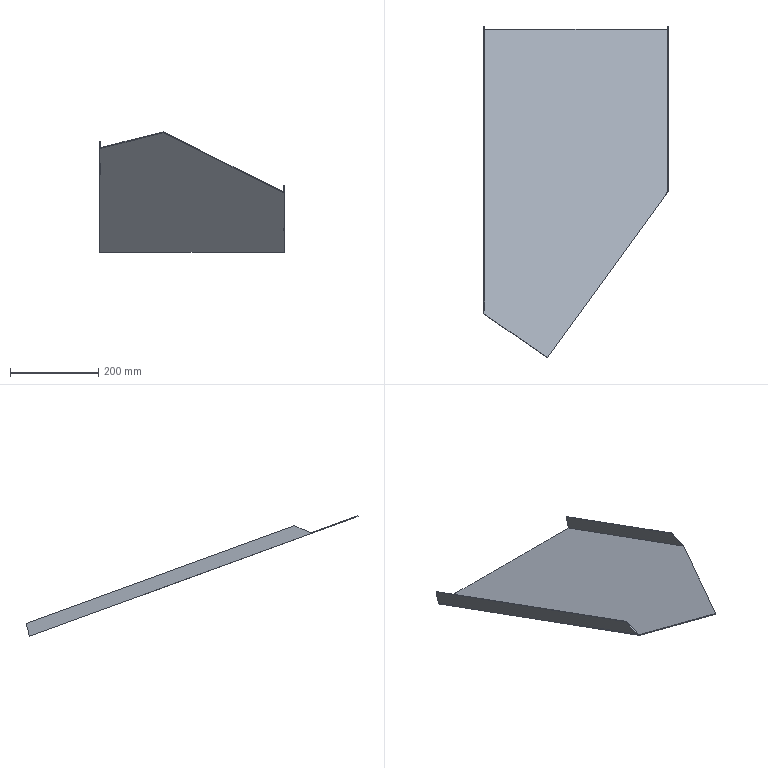Part | NX | features solid 2 | 1 solid | 13 faces | box 418.583 x 752.314 x 272.863 mm | volume 592956 mm3 | plane 12 | spline 1
STEP:
#1=CARTESIAN_POINT('',(-905.1,748.985,-499.373));
#2=VERTEX_POINT('',#1);
#3=CARTESIAN_POINT('',(-490.517,748.985,-499.373));
#4=VERTEX_POINT('',#3);
#5=CARTESIAN_POINT('',(-752.3,748.985,-499.373));
#6=DIRECTION('',(1.,0.,0.));
#7=VECTOR('',#6,1000.);
#8=LINE('',#5,#7);
#9=EDGE_CURVE('',#2,#4,#8,.T.);
#10=ORIENTED_EDGE('',*,*,#9,.F.);
#11=CARTESIAN_POINT('',(-905.1,111.413,-267.316));
#12=VERTEX_POINT('',#11);
#13=CARTESIAN_POINT('',(-905.1,3.724,-228.121));
#14=DIRECTION('',(0.,0.9397,-0.342));
#15=VECTOR('',#14,1000.);
#16=LINE('',#13,#15);
#17=EDGE_CURVE('',#12,#2,#16,.T.);
#18=ORIENTED_EDGE('',*,*,#17,.F.);
#19=CARTESIAN_POINT('',(-907.1,111.413,-267.316));
#20=VERTEX_POINT('',#19);
#21=CARTESIAN_POINT('',(-917.1,111.413,-267.316));
#22=DIRECTION('',(1.,0.,0.));
#23=VECTOR('',#22,1000.);
#24=LINE('',#21,#23);
#25=EDGE_CURVE('',#12,#20,#24,.F.);
#26=ORIENTED_EDGE('',*,*,#25,.T.);
#27=CARTESIAN_POINT('',(-907.1,104.555,-264.82));
#28=VERTEX_POINT('',#27);
#29=CARTESIAN_POINT('',(-907.1,3.724,-228.121));
#30=DIRECTION('',(0.,-0.9397,0.342));
#31=VECTOR('',#30,1000.);
#32=LINE('',#29,#31);
#33=EDGE_CURVE('',#20,#28,#32,.T.);
#34=ORIENTED_EDGE('',*,*,#33,.T.);
#35=CARTESIAN_POINT('',(-762.353,4.629,-228.45));
#36=VERTEX_POINT('',#35);
#37=CARTESIAN_POINT('',(-907.1,104.555,-264.82));
#38=CARTESIAN_POINT('',(-896.947,97.59,-262.285));
#39=CARTESIAN_POINT('',(-883.394,88.293,-258.901));
#40=CARTESIAN_POINT('',(-868.677,78.196,-255.226));
#41=CARTESIAN_POINT('',(-859.316,71.771,-252.888));
#42=CARTESIAN_POINT('',(-851.631,66.496,-250.968));
#43=CARTESIAN_POINT('',(-846.624,63.058,-249.716));
#44=CARTESIAN_POINT('',(-843.853,61.154,-249.023));
#45=CARTESIAN_POINT('',(-842.479,60.21,-248.68));
#46=CARTESIAN_POINT('',(-841.553,59.573,-248.448));
#47=CARTESIAN_POINT('',(-840.869,59.103,-248.277));
#48=CARTESIAN_POINT('',(-840.374,58.762,-248.153));
#49=CARTESIAN_POINT('',(-840.088,58.565,-248.081));
#50=CARTESIAN_POINT('',(-839.869,58.414,-248.026));
#51=CARTESIAN_POINT('',(-839.743,58.327,-247.994));
#52=CARTESIAN_POINT('',(-839.635,58.253,-247.967));
#53=CARTESIAN_POINT('',(-839.583,58.217,-247.954));
#54=CARTESIAN_POINT('',(-839.237,57.979,-247.868));
#55=CARTESIAN_POINT('',(-838.878,57.732,-247.778));
#56=CARTESIAN_POINT('',(-838.395,57.399,-247.656));
#57=CARTESIAN_POINT('',(-837.64,56.879,-247.467));
#58=CARTESIAN_POINT('',(-836.689,56.223,-247.229));
#59=CARTESIAN_POINT('',(-835.549,55.437,-246.943));
#60=CARTESIAN_POINT('',(-834.026,54.387,-246.56));
#61=CARTESIAN_POINT('',(-831.356,52.545,-245.89));
#62=CARTESIAN_POINT('',(-827.525,49.9,-244.927));
#63=CARTESIAN_POINT('',(-822.904,46.706,-243.765));
#64=CARTESIAN_POINT('',(-818.257,43.491,-242.595));
#65=CARTESIAN_POINT('',(-813.586,40.256,-241.417));
#66=CARTESIAN_POINT('',(-809.672,37.543,-240.43));
#67=CARTESIAN_POINT('',(-806.921,35.635,-239.735));
#68=CARTESIAN_POINT('',(-805.347,34.542,-239.337));
#69=CARTESIAN_POINT('',(-804.162,33.72,-239.038));
#70=CARTESIAN_POINT('',(-802.985,32.903,-238.741));
#71=CARTESIAN_POINT('',(-801.974,32.2,-238.485));
#72=CARTESIAN_POINT('',(-801.322,31.748,-238.32));
#73=CARTESIAN_POINT('',(-800.861,31.427,-238.204));
#74=CARTESIAN_POINT('',(-800.879,31.44,-238.208));
#75=CARTESIAN_POINT('',(-800.728,31.335,-238.17));
#76=CARTESIAN_POINT('',(-800.56,31.218,-238.127));
#77=CARTESIAN_POINT('',(-800.282,31.025,-238.057));
#78=CARTESIAN_POINT('',(-799.781,30.676,-237.93));
#79=CARTESIAN_POINT('',(-799.007,30.138,-237.735));
#80=CARTESIAN_POINT('',(-797.857,29.338,-237.443));
#81=CARTESIAN_POINT('',(-796.021,28.061,-236.978));
#82=CARTESIAN_POINT('',(-793.163,26.073,-236.255));
#83=CARTESIAN_POINT('',(-788.833,23.059,-235.158));
#84=CARTESIAN_POINT('',(-783.602,19.419,-233.833));
#85=CARTESIAN_POINT('',(-775.426,13.729,-231.762));
#86=CARTESIAN_POINT('',(-767.943,8.52,-229.866));
#87=CARTESIAN_POINT('',(-762.353,4.629,-228.45));
#88=B_SPLINE_CURVE_WITH_KNOTS('',3,(#37,#38,#39,#40,#41,#42,#43,#44,#45,#46,#47,#48,#49,#50,#51,#52,#53,#54,#55,#56,#57,#58,#59,#60,#61,#62,#63,#64,#65,#66,#67,#68,#69,#70,#71,#72,#73,#74,#75,#76,#77,#78,#79,#80,#81,#82,#83,#84,#85,#86,#87),.UNSPECIFIED.,.F.,.F.,(4,1,1,1,1,1,1,1,1,1,1,1,1,1,1,1,1,1,1,1,1,1,1,1,1,1,1,1,1,1,1,1,1,1,1,1,1,1,1,1,1,1,1,1,1,1,1,1,4),(0.03814,0.1584,0.2185,0.2786,0.3387,0.3988,0.4289,0.4439,0.459,0.474,0.4815,0.489,0.4928,0.4965,0.4984,0.5003,0.5022,0.504,0.5078,0.5116,0.5191,0.5266,0.5341,0.5491,0.5792,0.6092,0.6393,0.6694,0.6994,0.7144,0.722,0.7295,0.737,0.7445,0.7483,0.7501,0.752,0.7558,0.7595,0.767,0.7746,0.7896,0.8046,0.8197,0.8497,0.8798,0.9098,0.9399,1.),.UNSPECIFIED.);
#89=EDGE_CURVE('',#28,#36,#88,.T.);
#90=ORIENTED_EDGE('',*,*,#89,.T.);
#91=CARTESIAN_POINT('',(-488.517,382.431,-365.958));
#92=VERTEX_POINT('',#91);
#93=CARTESIAN_POINT('',(-846.744,-111.802,-186.072));
#94=DIRECTION('',(0.5629,0.7767,-0.2827));
#95=VECTOR('',#94,1000.);
#96=LINE('',#93,#95);
#97=EDGE_CURVE('',#92,#36,#96,.F.);
#98=ORIENTED_EDGE('',*,*,#97,.F.);
#99=CARTESIAN_POINT('',(-490.517,382.431,-365.958));
#100=VERTEX_POINT('',#99);
#101=CARTESIAN_POINT('',(-488.517,382.431,-365.958));
#102=DIRECTION('',(-1.,0.,0.));
#103=VECTOR('',#102,1000.);
#104=LINE('',#101,#103);
#105=EDGE_CURVE('',#92,#100,#104,.T.);
#106=ORIENTED_EDGE('',*,*,#105,.T.);
#107=CARTESIAN_POINT('',(-490.517,3.724,-228.121));
#108=DIRECTION('',(0.,0.9397,-0.342));
#109=VECTOR('',#108,1000.);
#110=LINE('',#107,#109);
#111=EDGE_CURVE('',#100,#4,#110,.T.);
#112=ORIENTED_EDGE('',*,*,#111,.T.);
#113=EDGE_LOOP('',(#10,#18,#26,#34,#90,#98,#106,#112));
#114=FACE_BOUND('',#113,.T.);
#115=CARTESIAN_POINT('',(-752.3,3.724,-228.121));
#116=DIRECTION('',(0.,0.342,0.9397));
#117=DIRECTION('',(1.,0.,0.));
#118=AXIS2_PLACEMENT_3D('',#115,#116,#117);
#119=PLANE('',#118);
#120=ADVANCED_FACE('',(#114),#119,.T.);
#121=CARTESIAN_POINT('',(-488.517,756.26,-472.224));
#122=VERTEX_POINT('',#121);
#123=CARTESIAN_POINT('',(-488.517,748.465,-501.312));
#124=VERTEX_POINT('',#123);
#125=CARTESIAN_POINT('',(-488.517,766.359,-434.531));
#126=DIRECTION('',(0.,-0.2588,-0.9659));
#127=VECTOR('',#126,1000.);
#128=LINE('',#125,#127);
#129=EDGE_CURVE('',#122,#124,#128,.T.);
#130=ORIENTED_EDGE('',*,*,#129,.F.);
#131=CARTESIAN_POINT('',(-488.517,418.318,-349.224));
#132=VERTEX_POINT('',#131);
#133=CARTESIAN_POINT('',(-488.517,392.007,-339.647));
#134=DIRECTION('',(0.,0.9397,-0.342));
#135=VECTOR('',#134,1000.);
#136=LINE('',#133,#135);
#137=EDGE_CURVE('',#132,#122,#136,.T.);
#138=ORIENTED_EDGE('',*,*,#137,.F.);
#139=CARTESIAN_POINT('',(-488.517,381.149,-366.556));
#140=DIRECTION('',(0.,0.9063,0.4226));
#141=VECTOR('',#140,1000.);
#142=LINE('',#139,#141);
#143=EDGE_CURVE('',#132,#92,#142,.F.);
#144=ORIENTED_EDGE('',*,*,#143,.T.);
#145=CARTESIAN_POINT('',(-488.517,381.746,-367.838));
#146=VERTEX_POINT('',#145);
#147=CARTESIAN_POINT('',(-488.517,381.746,-367.838));
#148=DIRECTION('',(0.,0.342,0.9397));
#149=VECTOR('',#148,1000.);
#150=LINE('',#147,#149);
#151=EDGE_CURVE('',#146,#92,#150,.T.);
#152=ORIENTED_EDGE('',*,*,#151,.F.);
#153=CARTESIAN_POINT('',(-488.517,3.04,-230.));
#154=DIRECTION('',(0.,0.9397,-0.342));
#155=VECTOR('',#154,1000.);
#156=LINE('',#153,#155);
#157=EDGE_CURVE('',#146,#124,#156,.T.);
#158=ORIENTED_EDGE('',*,*,#157,.T.);
#159=EDGE_LOOP('',(#130,#138,#144,#152,#158));
#160=FACE_BOUND('',#159,.T.);
#161=CARTESIAN_POINT('',(-488.517,3.04,-230.));
#162=DIRECTION('',(1.,0.,0.));
#163=DIRECTION('',(0.,1.,0.));
#164=AXIS2_PLACEMENT_3D('',#161,#162,#163);
#165=PLANE('',#164);
#166=ADVANCED_FACE('',(#160),#165,.T.);
#167=CARTESIAN_POINT('',(-907.1,147.301,-250.581));
#168=VERTEX_POINT('',#167);
#169=CARTESIAN_POINT('',(-907.1,756.26,-472.224));
#170=VERTEX_POINT('',#169);
#171=CARTESIAN_POINT('',(-907.1,120.99,-241.005));
#172=DIRECTION('',(0.,-0.9397,0.342));
#173=VECTOR('',#172,1000.);
#174=LINE('',#171,#173);
#175=EDGE_CURVE('',#168,#170,#174,.F.);
#176=ORIENTED_EDGE('',*,*,#175,.T.);
#177=CARTESIAN_POINT('',(-907.1,748.465,-501.312));
#178=VERTEX_POINT('',#177);
#179=CARTESIAN_POINT('',(-907.1,766.359,-434.531));
#180=DIRECTION('',(0.,-0.2588,-0.9659));
#181=VECTOR('',#180,1000.);
#182=LINE('',#179,#181);
#183=EDGE_CURVE('',#170,#178,#182,.T.);
#184=ORIENTED_EDGE('',*,*,#183,.T.);
#185=CARTESIAN_POINT('',(-907.1,103.871,-266.699));
#186=VERTEX_POINT('',#185);
#187=CARTESIAN_POINT('',(-907.1,3.04,-230.));
#188=DIRECTION('',(0.,0.9397,-0.342));
#189=VECTOR('',#188,1000.);
#190=LINE('',#187,#189);
#191=EDGE_CURVE('',#186,#178,#190,.T.);
#192=ORIENTED_EDGE('',*,*,#191,.F.);
#193=CARTESIAN_POINT('',(-907.1,104.213,-265.759));
#194=DIRECTION('',(0.,0.342,0.9397));
#195=VECTOR('',#194,1000.);
#196=LINE('',#193,#195);
#197=EDGE_CURVE('',#186,#28,#196,.T.);
#198=ORIENTED_EDGE('',*,*,#197,.T.);
#199=ORIENTED_EDGE('',*,*,#33,.F.);
#200=CARTESIAN_POINT('',(-907.1,147.301,-250.581));
#201=DIRECTION('',(0.,-0.9063,-0.4226));
#202=VECTOR('',#201,1000.);
#203=LINE('',#200,#202);
#204=EDGE_CURVE('',#20,#168,#203,.F.);
#205=ORIENTED_EDGE('',*,*,#204,.T.);
#206=EDGE_LOOP('',(#176,#184,#192,#198,#199,#205));
#207=FACE_BOUND('',#206,.T.);
#208=CARTESIAN_POINT('',(-907.1,3.04,-230.));
#209=DIRECTION('',(1.,0.,0.));
#210=DIRECTION('',(0.,0.,-1.));
#211=AXIS2_PLACEMENT_3D('',#208,#209,#210);
#212=PLANE('',#211);
#213=ADVANCED_FACE('',(#207),#212,.F.);
#214=ORIENTED_EDGE('',*,*,#89,.F.);
#215=ORIENTED_EDGE('',*,*,#197,.F.);
#216=CARTESIAN_POINT('',(-762.353,3.945,-230.329));
#217=VERTEX_POINT('',#216);
#218=CARTESIAN_POINT('',(-907.1,103.871,-266.699));
#219=CARTESIAN_POINT('',(-896.947,96.906,-264.164));
#220=CARTESIAN_POINT('',(-883.394,87.609,-260.781));
#221=CARTESIAN_POINT('',(-868.677,77.512,-257.105));
#222=CARTESIAN_POINT('',(-859.316,71.087,-254.767));
#223=CARTESIAN_POINT('',(-851.631,65.812,-252.847));
#224=CARTESIAN_POINT('',(-846.624,62.374,-251.596));
#225=CARTESIAN_POINT('',(-843.853,60.47,-250.903));
#226=CARTESIAN_POINT('',(-842.479,59.526,-250.559));
#227=CARTESIAN_POINT('',(-841.553,58.889,-250.327));
#228=CARTESIAN_POINT('',(-840.869,58.419,-250.156));
#229=CARTESIAN_POINT('',(-840.374,58.078,-250.032));
#230=CARTESIAN_POINT('',(-840.088,57.881,-249.96));
#231=CARTESIAN_POINT('',(-839.869,57.73,-249.906));
#232=CARTESIAN_POINT('',(-839.743,57.643,-249.874));
#233=CARTESIAN_POINT('',(-839.635,57.569,-249.847));
#234=CARTESIAN_POINT('',(-839.583,57.533,-249.834));
#235=CARTESIAN_POINT('',(-839.237,57.295,-249.747));
#236=CARTESIAN_POINT('',(-838.878,57.048,-249.657));
#237=CARTESIAN_POINT('',(-838.395,56.715,-249.536));
#238=CARTESIAN_POINT('',(-837.64,56.194,-249.347));
#239=CARTESIAN_POINT('',(-836.689,55.539,-249.108));
#240=CARTESIAN_POINT('',(-835.549,54.753,-248.822));
#241=CARTESIAN_POINT('',(-834.026,53.703,-248.44));
#242=CARTESIAN_POINT('',(-831.356,51.861,-247.769));
#243=CARTESIAN_POINT('',(-827.525,49.216,-246.807));
#244=CARTESIAN_POINT('',(-822.904,46.022,-245.644));
#245=CARTESIAN_POINT('',(-818.257,42.807,-244.474));
#246=CARTESIAN_POINT('',(-813.586,39.572,-243.296));
#247=CARTESIAN_POINT('',(-809.672,36.859,-242.309));
#248=CARTESIAN_POINT('',(-806.921,34.951,-241.614));
#249=CARTESIAN_POINT('',(-805.347,33.858,-241.217));
#250=CARTESIAN_POINT('',(-804.162,33.036,-240.917));
#251=CARTESIAN_POINT('',(-802.985,32.219,-240.62));
#252=CARTESIAN_POINT('',(-801.974,31.516,-240.364));
#253=CARTESIAN_POINT('',(-801.322,31.064,-240.2));
#254=CARTESIAN_POINT('',(-800.861,30.743,-240.083));
#255=CARTESIAN_POINT('',(-800.879,30.756,-240.088));
#256=CARTESIAN_POINT('',(-800.728,30.651,-240.049));
#257=CARTESIAN_POINT('',(-800.56,30.534,-240.007));
#258=CARTESIAN_POINT('',(-800.282,30.341,-239.937));
#259=CARTESIAN_POINT('',(-799.781,29.992,-239.81));
#260=CARTESIAN_POINT('',(-799.007,29.454,-239.614));
#261=CARTESIAN_POINT('',(-797.857,28.654,-239.323));
#262=CARTESIAN_POINT('',(-796.021,27.377,-238.858));
#263=CARTESIAN_POINT('',(-793.163,25.389,-238.134));
#264=CARTESIAN_POINT('',(-788.833,22.375,-237.037));
#265=CARTESIAN_POINT('',(-783.602,18.735,-235.712));
#266=CARTESIAN_POINT('',(-775.426,13.045,-233.641));
#267=CARTESIAN_POINT('',(-767.943,7.836,-231.745));
#268=CARTESIAN_POINT('',(-762.353,3.945,-230.329));
#269=B_SPLINE_CURVE_WITH_KNOTS('',3,(#218,#219,#220,#221,#222,#223,#224,#225,#226,#227,#228,#229,#230,#231,#232,#233,#234,#235,#236,#237,#238,#239,#240,#241,#242,#243,#244,#245,#246,#247,#248,#249,#250,#251,#252,#253,#254,#255,#256,#257,#258,#259,#260,#261,#262,#263,#264,#265,#266,#267,#268),.UNSPECIFIED.,.F.,.F.,(4,1,1,1,1,1,1,1,1,1,1,1,1,1,1,1,1,1,1,1,1,1,1,1,1,1,1,1,1,1,1,1,1,1,1,1,1,1,1,1,1,1,1,1,1,1,1,1,4),(0.03814,0.1584,0.2185,0.2786,0.3387,0.3988,0.4289,0.4439,0.459,0.474,0.4815,0.489,0.4928,0.4965,0.4984,0.5003,0.5022,0.504,0.5078,0.5116,0.5191,0.5266,0.5341,0.5491,0.5792,0.6092,0.6393,0.6694,0.6994,0.7144,0.722,0.7295,0.737,0.7445,0.7483,0.7501,0.752,0.7558,0.7595,0.767,0.7746,0.7896,0.8046,0.8197,0.8497,0.8798,0.9098,0.9399,1.),.UNSPECIFIED.);
#270=EDGE_CURVE('',#186,#217,#269,.T.);
#271=ORIENTED_EDGE('',*,*,#270,.T.);
#272=CARTESIAN_POINT('',(-762.353,3.945,-230.329));
#273=CARTESIAN_POINT('',(-762.353,4.173,-229.703));
#274=CARTESIAN_POINT('',(-762.353,4.401,-229.076));
#275=CARTESIAN_POINT('',(-762.353,4.629,-228.45));
#276=B_SPLINE_CURVE_WITH_KNOTS('',3,(#272,#273,#274,#275),.UNSPECIFIED.,.F.,.F.,(4,4),(0.,1.),.UNSPECIFIED.);
#277=EDGE_CURVE('',#217,#36,#276,.T.);
#278=ORIENTED_EDGE('',*,*,#277,.T.);
#279=EDGE_LOOP('',(#214,#215,#271,#278));
#280=FACE_BOUND('',#279,.T.);
#281=CARTESIAN_POINT('',(-907.1,103.871,-266.699));
#282=CARTESIAN_POINT('',(-907.1,104.555,-264.82));
#283=CARTESIAN_POINT('',(-886.794,89.942,-261.63));
#284=CARTESIAN_POINT('',(-886.794,90.626,-259.75));
#285=CARTESIAN_POINT('',(-867.,76.362,-256.687));
#286=CARTESIAN_POINT('',(-867.,77.047,-254.808));
#287=CARTESIAN_POINT('',(-851.631,65.812,-252.847));
#288=CARTESIAN_POINT('',(-851.631,66.496,-250.968));
#289=CARTESIAN_POINT('',(-846.624,62.374,-251.596));
#290=CARTESIAN_POINT('',(-846.624,63.058,-249.716));
#291=CARTESIAN_POINT('',(-843.853,60.47,-250.903));
#292=CARTESIAN_POINT('',(-843.853,61.154,-249.023));
#293=CARTESIAN_POINT('',(-842.479,59.526,-250.559));
#294=CARTESIAN_POINT('',(-842.479,60.21,-248.68));
#295=CARTESIAN_POINT('',(-841.553,58.889,-250.327));
#296=CARTESIAN_POINT('',(-841.553,59.573,-248.448));
#297=CARTESIAN_POINT('',(-840.869,58.419,-250.156));
#298=CARTESIAN_POINT('',(-840.869,59.103,-248.277));
#299=CARTESIAN_POINT('',(-840.374,58.078,-250.032));
#300=CARTESIAN_POINT('',(-840.374,58.762,-248.153));
#301=CARTESIAN_POINT('',(-840.088,57.881,-249.96));
#302=CARTESIAN_POINT('',(-840.088,58.565,-248.081));
#303=CARTESIAN_POINT('',(-839.869,57.73,-249.906));
#304=CARTESIAN_POINT('',(-839.869,58.414,-248.026));
#305=CARTESIAN_POINT('',(-839.743,57.643,-249.874));
#306=CARTESIAN_POINT('',(-839.743,58.327,-247.994));
#307=CARTESIAN_POINT('',(-839.635,57.569,-249.847));
#308=CARTESIAN_POINT('',(-839.635,58.253,-247.967));
#309=CARTESIAN_POINT('',(-839.583,57.533,-249.834));
#310=CARTESIAN_POINT('',(-839.583,58.217,-247.954));
#311=CARTESIAN_POINT('',(-839.237,57.295,-249.747));
#312=CARTESIAN_POINT('',(-839.237,57.979,-247.868));
#313=CARTESIAN_POINT('',(-838.878,57.048,-249.657));
#314=CARTESIAN_POINT('',(-838.878,57.732,-247.778));
#315=CARTESIAN_POINT('',(-838.395,56.715,-249.536));
#316=CARTESIAN_POINT('',(-838.395,57.399,-247.656));
#317=CARTESIAN_POINT('',(-837.64,56.194,-249.347));
#318=CARTESIAN_POINT('',(-837.64,56.879,-247.467));
#319=CARTESIAN_POINT('',(-836.689,55.539,-249.108));
#320=CARTESIAN_POINT('',(-836.689,56.223,-247.229));
#321=CARTESIAN_POINT('',(-835.549,54.753,-248.822));
#322=CARTESIAN_POINT('',(-835.549,55.437,-246.943));
#323=CARTESIAN_POINT('',(-834.026,53.703,-248.44));
#324=CARTESIAN_POINT('',(-834.026,54.387,-246.56));
#325=CARTESIAN_POINT('',(-831.356,51.861,-247.769));
#326=CARTESIAN_POINT('',(-831.356,52.545,-245.89));
#327=CARTESIAN_POINT('',(-825.993,48.158,-246.422));
#328=CARTESIAN_POINT('',(-825.993,48.842,-244.542));
#329=CARTESIAN_POINT('',(-819.814,43.886,-244.867));
#330=CARTESIAN_POINT('',(-819.814,44.57,-242.987));
#331=CARTESIAN_POINT('',(-813.586,39.572,-243.296));
#332=CARTESIAN_POINT('',(-813.586,40.256,-241.417));
#333=CARTESIAN_POINT('',(-809.672,36.859,-242.309));
#334=CARTESIAN_POINT('',(-809.672,37.543,-240.43));
#335=CARTESIAN_POINT('',(-806.921,34.951,-241.614));
#336=CARTESIAN_POINT('',(-806.921,35.635,-239.735));
#337=CARTESIAN_POINT('',(-805.347,33.858,-241.217));
#338=CARTESIAN_POINT('',(-805.347,34.542,-239.337));
#339=CARTESIAN_POINT('',(-804.162,33.036,-240.917));
#340=CARTESIAN_POINT('',(-804.162,33.72,-239.038));
#341=CARTESIAN_POINT('',(-802.985,32.219,-240.62));
#342=CARTESIAN_POINT('',(-802.985,32.903,-238.741));
#343=CARTESIAN_POINT('',(-801.974,31.516,-240.364));
#344=CARTESIAN_POINT('',(-801.974,32.2,-238.485));
#345=CARTESIAN_POINT('',(-801.322,31.064,-240.2));
#346=CARTESIAN_POINT('',(-801.322,31.748,-238.32));
#347=CARTESIAN_POINT('',(-800.861,30.743,-240.083));
#348=CARTESIAN_POINT('',(-800.861,31.427,-238.204));
#349=CARTESIAN_POINT('',(-800.879,30.756,-240.088));
#350=CARTESIAN_POINT('',(-800.879,31.44,-238.208));
#351=CARTESIAN_POINT('',(-800.728,30.651,-240.049));
#352=CARTESIAN_POINT('',(-800.728,31.335,-238.17));
#353=CARTESIAN_POINT('',(-800.56,30.534,-240.007));
#354=CARTESIAN_POINT('',(-800.56,31.218,-238.127));
#355=CARTESIAN_POINT('',(-800.282,30.341,-239.937));
#356=CARTESIAN_POINT('',(-800.282,31.025,-238.057));
#357=CARTESIAN_POINT('',(-799.781,29.992,-239.81));
#358=CARTESIAN_POINT('',(-799.781,30.676,-237.93));
#359=CARTESIAN_POINT('',(-799.007,29.454,-239.614));
#360=CARTESIAN_POINT('',(-799.007,30.138,-237.735));
#361=CARTESIAN_POINT('',(-797.857,28.654,-239.323));
#362=CARTESIAN_POINT('',(-797.857,29.338,-237.443));
#363=CARTESIAN_POINT('',(-796.021,27.377,-238.858));
#364=CARTESIAN_POINT('',(-796.021,28.061,-236.978));
#365=CARTESIAN_POINT('',(-793.163,25.389,-238.134));
#366=CARTESIAN_POINT('',(-793.163,26.073,-236.255));
#367=CARTESIAN_POINT('',(-788.833,22.375,-237.037));
#368=CARTESIAN_POINT('',(-788.833,23.059,-235.158));
#369=CARTESIAN_POINT('',(-783.602,18.735,-235.712));
#370=CARTESIAN_POINT('',(-783.602,19.419,-233.833));
#371=CARTESIAN_POINT('',(-775.426,13.045,-233.641));
#372=CARTESIAN_POINT('',(-775.426,13.729,-231.762));
#373=CARTESIAN_POINT('',(-767.943,7.836,-231.745));
#374=CARTESIAN_POINT('',(-767.943,8.52,-229.866));
#375=CARTESIAN_POINT('',(-762.353,3.945,-230.329));
#376=CARTESIAN_POINT('',(-762.353,4.629,-228.45));
#377=B_SPLINE_SURFACE_WITH_KNOTS('',3,1,((#281,#282),(#283,#284),(#285,#286),(#287,#288),(#289,#290),(#291,#292),(#293,#294),(#295,#296),(#297,#298),(#299,#300),(#301,#302),(#303,#304),(#305,#306),(#307,#308),(#309,#310),(#311,#312),(#313,#314),(#315,#316),(#317,#318),(#319,#320),(#321,#322),(#323,#324),(#325,#326),(#327,#328),(#329,#330),(#331,#332),(#333,#334),(#335,#336),(#337,#338),(#339,#340),(#341,#342),(#343,#344),(#345,#346),(#347,#348),(#349,#350),(#351,#352),(#353,#354),(#355,#356),(#357,#358),(#359,#360),(#361,#362),(#363,#364),(#365,#366),(#367,#368),(#369,#370),(#371,#372),(#373,#374),(#375,#376)),.UNSPECIFIED.,.F.,.F.,.F.,(4,1,1,1,1,1,1,1,1,1,1,1,1,1,1,1,1,1,1,1,1,1,1,1,1,1,1,1,1,1,1,1,1,1,1,1,1,1,1,1,1,1,1,1,1,4),(2,2),(0.03814,0.2786,0.3387,0.3988,0.4289,0.4439,0.459,0.474,0.4815,0.489,0.4928,0.4965,0.4984,0.5003,0.5022,0.504,0.5078,0.5116,0.5191,0.5266,0.5341,0.5491,0.5792,0.6393,0.6694,0.6994,0.7144,0.722,0.7295,0.737,0.7445,0.7483,0.7501,0.752,0.7558,0.7595,0.767,0.7746,0.7896,0.8046,0.8197,0.8497,0.8798,0.9098,0.9399,1.),(0.,1.),.UNSPECIFIED.);
#378=ADVANCED_FACE('',(#280),#377,.T.);
#379=ORIENTED_EDGE('',*,*,#97,.T.);
#380=ORIENTED_EDGE('',*,*,#277,.F.);
#381=CARTESIAN_POINT('',(-846.744,-112.486,-187.952));
#382=DIRECTION('',(0.5629,0.7767,-0.2827));
#383=VECTOR('',#382,1000.);
#384=LINE('',#381,#383);
#385=EDGE_CURVE('',#146,#217,#384,.F.);
#386=ORIENTED_EDGE('',*,*,#385,.F.);
#387=ORIENTED_EDGE('',*,*,#151,.T.);
#388=EDGE_LOOP('',(#379,#380,#386,#387));
#389=FACE_BOUND('',#388,.T.);
#390=CARTESIAN_POINT('',(-846.744,-112.486,-187.952));
#391=DIRECTION('',(-0.8265,0.529,-0.1925));
#392=DIRECTION('',(-0.5391,-0.8423,0.));
#393=AXIS2_PLACEMENT_3D('',#390,#391,#392);
#394=PLANE('',#393);
#395=ADVANCED_FACE('',(#389),#394,.F.);
#396=ORIENTED_EDGE('',*,*,#191,.T.);
#397=CARTESIAN_POINT('',(-752.3,748.465,-501.312));
#398=DIRECTION('',(1.,0.,0.));
#399=VECTOR('',#398,1000.);
#400=LINE('',#397,#399);
#401=EDGE_CURVE('',#178,#124,#400,.T.);
#402=ORIENTED_EDGE('',*,*,#401,.T.);
#403=ORIENTED_EDGE('',*,*,#157,.F.);
#404=ORIENTED_EDGE('',*,*,#385,.T.);
#405=ORIENTED_EDGE('',*,*,#270,.F.);
#406=EDGE_LOOP('',(#396,#402,#403,#404,#405));
#407=FACE_BOUND('',#406,.T.);
#408=CARTESIAN_POINT('',(-752.3,3.04,-230.));
#409=DIRECTION('',(0.,0.342,0.9397));
#410=DIRECTION('',(1.,0.,0.));
#411=AXIS2_PLACEMENT_3D('',#408,#409,#410);
#412=PLANE('',#411);
#413=ADVANCED_FACE('',(#407),#412,.F.);
#414=CARTESIAN_POINT('',(-490.517,418.318,-349.224));
#415=VERTEX_POINT('',#414);
#416=CARTESIAN_POINT('',(-490.517,756.26,-472.224));
#417=VERTEX_POINT('',#416);
#418=CARTESIAN_POINT('',(-490.517,392.007,-339.647));
#419=DIRECTION('',(0.,0.9397,-0.342));
#420=VECTOR('',#419,1000.);
#421=LINE('',#418,#420);
#422=EDGE_CURVE('',#415,#417,#421,.T.);
#423=ORIENTED_EDGE('',*,*,#422,.T.);
#424=CARTESIAN_POINT('',(-490.517,757.268,-468.459));
#425=DIRECTION('',(0.,-0.2588,-0.9659));
#426=VECTOR('',#425,1000.);
#427=LINE('',#424,#426);
#428=EDGE_CURVE('',#417,#4,#427,.T.);
#429=ORIENTED_EDGE('',*,*,#428,.T.);
#430=ORIENTED_EDGE('',*,*,#111,.F.);
#431=CARTESIAN_POINT('',(-490.517,382.431,-365.958));
#432=DIRECTION('',(0.,-0.9063,-0.4226));
#433=VECTOR('',#432,1000.);
#434=LINE('',#431,#433);
#435=EDGE_CURVE('',#100,#415,#434,.F.);
#436=ORIENTED_EDGE('',*,*,#435,.T.);
#437=EDGE_LOOP('',(#423,#429,#430,#436));
#438=FACE_BOUND('',#437,.T.);
#439=CARTESIAN_POINT('',(-490.517,381.746,-367.838));
#440=DIRECTION('',(1.,0.,0.));
#441=DIRECTION('',(0.,1.,0.));
#442=AXIS2_PLACEMENT_3D('',#439,#440,#441);
#443=PLANE('',#442);
#444=ADVANCED_FACE('',(#438),#443,.F.);
#445=ORIENTED_EDGE('',*,*,#137,.T.);
#446=CARTESIAN_POINT('',(-488.517,756.26,-472.224));
#447=DIRECTION('',(-1.,0.,0.));
#448=VECTOR('',#447,1000.);
#449=LINE('',#446,#448);
#450=EDGE_CURVE('',#122,#417,#449,.T.);
#451=ORIENTED_EDGE('',*,*,#450,.T.);
#452=ORIENTED_EDGE('',*,*,#422,.F.);
#453=CARTESIAN_POINT('',(-488.517,418.318,-349.224));
#454=DIRECTION('',(1.,0.,0.));
#455=VECTOR('',#454,1000.);
#456=LINE('',#453,#455);
#457=EDGE_CURVE('',#415,#132,#456,.T.);
#458=ORIENTED_EDGE('',*,*,#457,.T.);
#459=EDGE_LOOP('',(#445,#451,#452,#458));
#460=FACE_BOUND('',#459,.T.);
#461=CARTESIAN_POINT('',(-488.517,392.007,-339.647));
#462=DIRECTION('',(0.,-0.342,-0.9397));
#463=DIRECTION('',(0.,0.9397,-0.342));
#464=AXIS2_PLACEMENT_3D('',#461,#462,#463);
#465=PLANE('',#464);
#466=ADVANCED_FACE('',(#460),#465,.F.);
#467=ORIENTED_EDGE('',*,*,#143,.F.);
#468=ORIENTED_EDGE('',*,*,#457,.F.);
#469=ORIENTED_EDGE('',*,*,#435,.F.);
#470=ORIENTED_EDGE('',*,*,#105,.F.);
#471=EDGE_LOOP('',(#467,#468,#469,#470));
#472=FACE_BOUND('',#471,.T.);
#473=CARTESIAN_POINT('',(-488.517,382.431,-365.958));
#474=DIRECTION('',(0.,0.4226,-0.9063));
#475=DIRECTION('',(0.,0.9063,0.4226));
#476=AXIS2_PLACEMENT_3D('',#473,#474,#475);
#477=PLANE('',#476);
#478=ADVANCED_FACE('',(#472),#477,.F.);
#479=CARTESIAN_POINT('',(-905.1,756.26,-472.224));
#480=VERTEX_POINT('',#479);
#481=CARTESIAN_POINT('',(-905.1,763.774,-444.178));
#482=DIRECTION('',(0.,-0.2588,-0.9659));
#483=VECTOR('',#482,1000.);
#484=LINE('',#481,#483);
#485=EDGE_CURVE('',#480,#2,#484,.T.);
#486=ORIENTED_EDGE('',*,*,#485,.F.);
#487=CARTESIAN_POINT('',(-905.1,147.301,-250.581));
#488=VERTEX_POINT('',#487);
#489=CARTESIAN_POINT('',(-905.1,120.99,-241.005));
#490=DIRECTION('',(0.,-0.9397,0.342));
#491=VECTOR('',#490,1000.);
#492=LINE('',#489,#491);
#493=EDGE_CURVE('',#488,#480,#492,.F.);
#494=ORIENTED_EDGE('',*,*,#493,.F.);
#495=CARTESIAN_POINT('',(-905.1,110.132,-267.914));
#496=DIRECTION('',(0.,0.9063,0.4226));
#497=VECTOR('',#496,1000.);
#498=LINE('',#495,#497);
#499=EDGE_CURVE('',#488,#12,#498,.F.);
#500=ORIENTED_EDGE('',*,*,#499,.T.);
#501=ORIENTED_EDGE('',*,*,#17,.T.);
#502=EDGE_LOOP('',(#486,#494,#500,#501));
#503=FACE_BOUND('',#502,.T.);
#504=CARTESIAN_POINT('',(-905.1,110.729,-269.196));
#505=DIRECTION('',(1.,0.,0.));
#506=DIRECTION('',(0.,0.,-1.));
#507=AXIS2_PLACEMENT_3D('',#504,#505,#506);
#508=PLANE('',#507);
#509=ADVANCED_FACE('',(#503),#508,.T.);
#510=CARTESIAN_POINT('',(-917.1,756.26,-472.224));
#511=DIRECTION('',(-1.,0.,0.));
#512=VECTOR('',#511,1000.);
#513=LINE('',#510,#512);
#514=EDGE_CURVE('',#170,#480,#513,.F.);
#515=ORIENTED_EDGE('',*,*,#514,.F.);
#516=ORIENTED_EDGE('',*,*,#175,.F.);
#517=CARTESIAN_POINT('',(-917.1,147.301,-250.581));
#518=DIRECTION('',(-1.,0.,0.));
#519=VECTOR('',#518,1000.);
#520=LINE('',#517,#519);
#521=EDGE_CURVE('',#168,#488,#520,.F.);
#522=ORIENTED_EDGE('',*,*,#521,.T.);
#523=ORIENTED_EDGE('',*,*,#493,.T.);
#524=EDGE_LOOP('',(#515,#516,#522,#523));
#525=FACE_BOUND('',#524,.T.);
#526=CARTESIAN_POINT('',(-917.1,120.99,-241.005));
#527=DIRECTION('',(0.,-0.342,-0.9397));
#528=DIRECTION('',(0.,0.9397,-0.342));
#529=AXIS2_PLACEMENT_3D('',#526,#527,#528);
#530=PLANE('',#529);
#531=ADVANCED_FACE('',(#525),#530,.F.);
#532=ORIENTED_EDGE('',*,*,#204,.F.);
#533=ORIENTED_EDGE('',*,*,#25,.F.);
#534=ORIENTED_EDGE('',*,*,#499,.F.);
#535=ORIENTED_EDGE('',*,*,#521,.F.);
#536=EDGE_LOOP('',(#532,#533,#534,#535));
#537=FACE_BOUND('',#536,.T.);
#538=CARTESIAN_POINT('',(-917.1,147.301,-250.581));
#539=DIRECTION('',(0.,0.4226,-0.9063));
#540=DIRECTION('',(0.,0.9063,0.4226));
#541=AXIS2_PLACEMENT_3D('',#538,#539,#540);
#542=PLANE('',#541);
#543=ADVANCED_FACE('',(#537),#542,.F.);
#544=ORIENTED_EDGE('',*,*,#450,.F.);
#545=ORIENTED_EDGE('',*,*,#129,.T.);
#546=ORIENTED_EDGE('',*,*,#401,.F.);
#547=ORIENTED_EDGE('',*,*,#183,.F.);
#548=ORIENTED_EDGE('',*,*,#514,.T.);
#549=ORIENTED_EDGE('',*,*,#485,.T.);
#550=ORIENTED_EDGE('',*,*,#9,.T.);
#551=ORIENTED_EDGE('',*,*,#428,.F.);
#552=EDGE_LOOP('',(#544,#545,#546,#547,#548,#549,#550,#551));
#553=FACE_BOUND('',#552,.T.);
#554=CARTESIAN_POINT('',(-917.1,750.519,-493.649));
#555=DIRECTION('',(0.,-0.9659,0.2588));
#556=DIRECTION('',(0.,-0.2588,-0.9659));
#557=AXIS2_PLACEMENT_3D('',#554,#555,#556);
#558=PLANE('',#557);
#559=ADVANCED_FACE('',(#553),#558,.F.);
#560=CLOSED_SHELL('',(#120,#166,#213,#378,#395,#413,#444,#466,#478,#509,#531,#543,#559));
#561=MANIFOLD_SOLID_BREP('',#560);
#562=(LENGTH_UNIT()NAMED_UNIT(*)SI_UNIT(.MILLI.,.METRE.));
#563=UNCERTAINTY_MEASURE_WITH_UNIT(LENGTH_MEASURE(0.0508),#562,'','');
#564=(NAMED_UNIT(*)PLANE_ANGLE_UNIT()SI_UNIT($,.RADIAN.));
#565=(NAMED_UNIT(*)SI_UNIT($,.STERADIAN.)SOLID_ANGLE_UNIT());
#566=(GEOMETRIC_REPRESENTATION_CONTEXT(3)GLOBAL_UNCERTAINTY_ASSIGNED_CONTEXT((#563))GLOBAL_UNIT_ASSIGNED_CONTEXT((#562,#564,#565))REPRESENTATION_CONTEXT('',''));
#567=ADVANCED_BREP_SHAPE_REPRESENTATION('',(#561),#566);